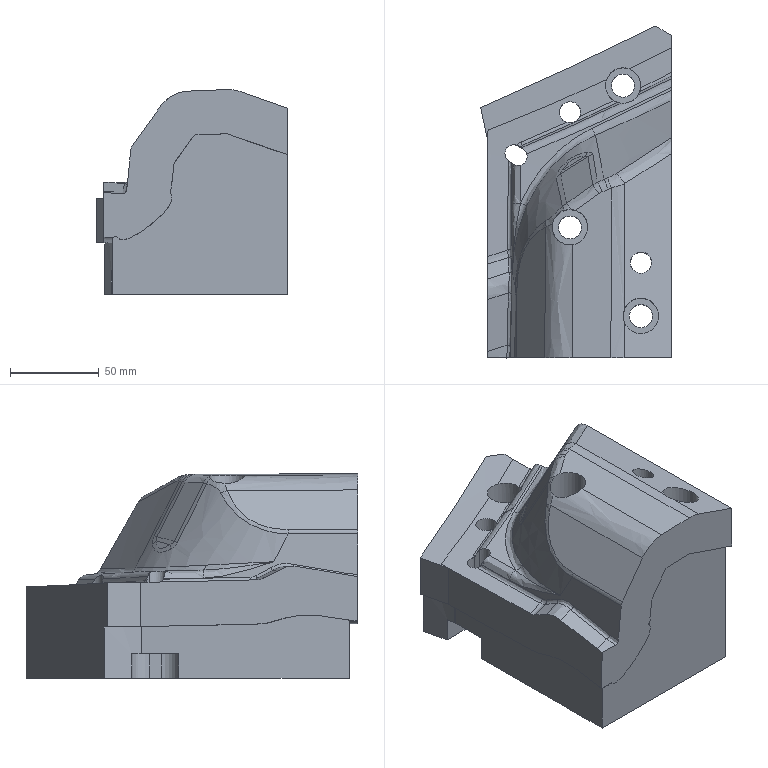Part | NX | features solid 2 | 1 solid | 98 faces | box 107.621 x 187.208 x 115.55 mm | volume 1315298 mm3 | spline 65 | plane 19 | cylinder 14 | commonest cylinder face diameters 20 x5 13 x3 10.1 x2 12 x2 14.1 x2